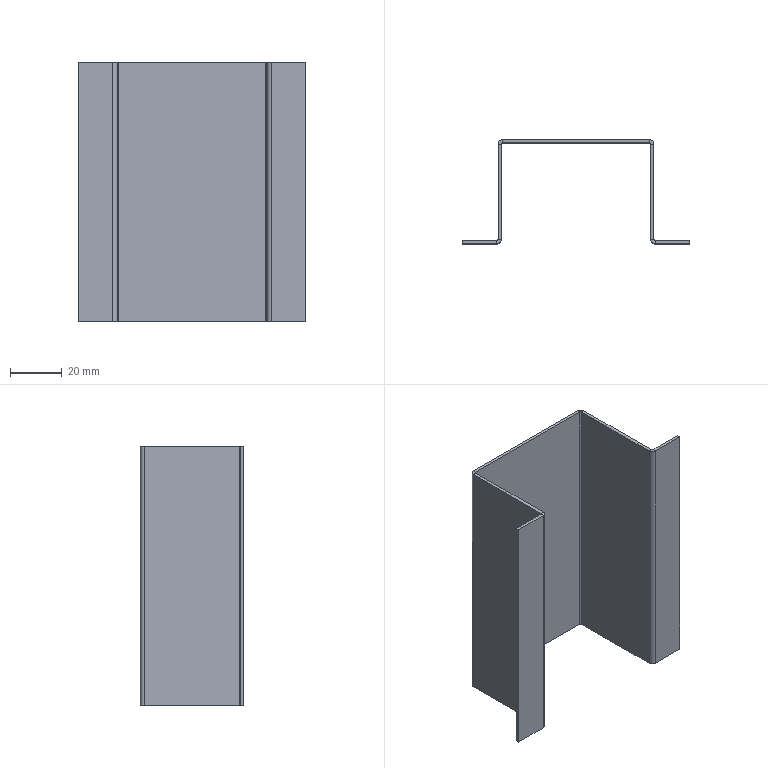Part | SolidWorks | features EdgeFlange 2, FlatPattern 1, SMBaseFlange 1, SheetMetal 1 | 1 solid | 38 faces | box 87.6 x 40 x 100 mm | volume 19608 mm3 | plane 30 | cylinder 8 | commonest cylinder face diameters 0.9 x4 3.3 x4
STEP:
#1=CARTESIAN_POINT('',(-19.132,-0.45,79.221));
#2=VERTEX_POINT('',#1);
#3=CARTESIAN_POINT('',(-19.132,-37.15,79.221));
#4=VERTEX_POINT('',#3);
#5=CARTESIAN_POINT('',(-19.132,-38.8,79.221));
#6=DIRECTION('',(0.,-1.,0.));
#7=VECTOR('',#6,1000.);
#8=LINE('',#5,#7);
#9=EDGE_CURVE('',#2,#4,#8,.T.);
#10=ORIENTED_EDGE('',*,*,#9,.T.);
#11=CARTESIAN_POINT('',(-17.932,-37.15,79.221));
#12=VERTEX_POINT('',#11);
#13=CARTESIAN_POINT('',(-19.132,-37.15,79.221));
#14=DIRECTION('',(1.,0.,0.));
#15=VECTOR('',#14,1000.);
#16=LINE('',#13,#15);
#17=EDGE_CURVE('',#4,#12,#16,.T.);
#18=ORIENTED_EDGE('',*,*,#17,.T.);
#19=CARTESIAN_POINT('',(-17.932,-0.45,79.221));
#20=VERTEX_POINT('',#19);
#21=CARTESIAN_POINT('',(-17.932,0.,79.221));
#22=DIRECTION('',(0.,-1.,0.));
#23=VECTOR('',#22,1000.);
#24=LINE('',#21,#23);
#25=EDGE_CURVE('',#20,#12,#24,.T.);
#26=ORIENTED_EDGE('',*,*,#25,.F.);
#27=CARTESIAN_POINT('',(-19.132,-0.45,79.221));
#28=DIRECTION('',(-1.,0.,0.));
#29=VECTOR('',#28,1000.);
#30=LINE('',#27,#29);
#31=EDGE_CURVE('',#20,#2,#30,.T.);
#32=ORIENTED_EDGE('',*,*,#31,.T.);
#33=EDGE_LOOP('',(#10,#18,#26,#32));
#34=FACE_OUTER_BOUND('',#33,.T.);
#35=CARTESIAN_POINT('',(-19.132,-38.8,79.221));
#36=DIRECTION('',(0.,0.,1.));
#37=DIRECTION('',(1.,0.,0.));
#38=AXIS2_PLACEMENT_3D('',#35,#36,#37);
#39=PLANE('',#38);
#40=ADVANCED_FACE('',(#34),#39,.T.);
#41=CARTESIAN_POINT('',(-19.132,-37.15,-20.779));
#42=VERTEX_POINT('',#41);
#43=CARTESIAN_POINT('',(-19.132,-0.45,-20.779));
#44=VERTEX_POINT('',#43);
#45=CARTESIAN_POINT('',(-19.132,0.,-20.779));
#46=DIRECTION('',(0.,1.,0.));
#47=VECTOR('',#46,1000.);
#48=LINE('',#45,#47);
#49=EDGE_CURVE('',#42,#44,#48,.T.);
#50=ORIENTED_EDGE('',*,*,#49,.F.);
#51=CARTESIAN_POINT('',(-19.132,-37.15,79.221));
#52=DIRECTION('',(0.,0.,-1.));
#53=VECTOR('',#52,1000.);
#54=LINE('',#51,#53);
#55=EDGE_CURVE('',#4,#42,#54,.T.);
#56=ORIENTED_EDGE('',*,*,#55,.F.);
#57=ORIENTED_EDGE('',*,*,#9,.F.);
#58=CARTESIAN_POINT('',(-19.132,-0.45,-20.779));
#59=DIRECTION('',(0.,0.,-1.));
#60=VECTOR('',#59,1000.);
#61=LINE('',#58,#60);
#62=EDGE_CURVE('',#2,#44,#61,.T.);
#63=ORIENTED_EDGE('',*,*,#62,.T.);
#64=EDGE_LOOP('',(#50,#56,#57,#63));
#65=FACE_OUTER_BOUND('',#64,.T.);
#66=CARTESIAN_POINT('',(-19.132,0.,-20.779));
#67=DIRECTION('',(-1.,0.,0.));
#68=DIRECTION('',(0.,-1.,0.));
#69=AXIS2_PLACEMENT_3D('',#66,#67,#68);
#70=PLANE('',#69);
#71=ADVANCED_FACE('',(#65),#70,.T.);
#72=CARTESIAN_POINT('',(-17.932,-37.15,-20.779));
#73=VERTEX_POINT('',#72);
#74=CARTESIAN_POINT('',(-17.932,-37.15,79.221));
#75=DIRECTION('',(0.,0.,-1.));
#76=VECTOR('',#75,1000.);
#77=LINE('',#74,#76);
#78=EDGE_CURVE('',#12,#73,#77,.T.);
#79=ORIENTED_EDGE('',*,*,#78,.T.);
#80=CARTESIAN_POINT('',(-17.932,-0.45,-20.779));
#81=VERTEX_POINT('',#80);
#82=CARTESIAN_POINT('',(-17.932,0.,-20.779));
#83=DIRECTION('',(0.,1.,0.));
#84=VECTOR('',#83,1000.);
#85=LINE('',#82,#84);
#86=EDGE_CURVE('',#73,#81,#85,.T.);
#87=ORIENTED_EDGE('',*,*,#86,.T.);
#88=CARTESIAN_POINT('',(-17.932,-0.45,79.221));
#89=DIRECTION('',(0.,0.,-1.));
#90=VECTOR('',#89,1000.);
#91=LINE('',#88,#90);
#92=EDGE_CURVE('',#20,#81,#91,.T.);
#93=ORIENTED_EDGE('',*,*,#92,.F.);
#94=ORIENTED_EDGE('',*,*,#25,.T.);
#95=EDGE_LOOP('',(#79,#87,#93,#94));
#96=FACE_OUTER_BOUND('',#95,.T.);
#97=CARTESIAN_POINT('',(-17.932,0.,-20.779));
#98=DIRECTION('',(-1.,0.,0.));
#99=DIRECTION('',(0.,-1.,0.));
#100=AXIS2_PLACEMENT_3D('',#97,#98,#99);
#101=PLANE('',#100);
#102=ADVANCED_FACE('',(#96),#101,.F.);
#103=CARTESIAN_POINT('',(40.868,-0.45,-20.779));
#104=VERTEX_POINT('',#103);
#105=CARTESIAN_POINT('',(40.868,-37.15,-20.779));
#106=VERTEX_POINT('',#105);
#107=CARTESIAN_POINT('',(40.868,0.,-20.779));
#108=DIRECTION('',(0.,-1.,0.));
#109=VECTOR('',#108,1000.);
#110=LINE('',#107,#109);
#111=EDGE_CURVE('',#104,#106,#110,.T.);
#112=ORIENTED_EDGE('',*,*,#111,.T.);
#113=CARTESIAN_POINT('',(39.668,-37.15,-20.779));
#114=VERTEX_POINT('',#113);
#115=CARTESIAN_POINT('',(40.868,-37.15,-20.779));
#116=DIRECTION('',(-1.,0.,0.));
#117=VECTOR('',#116,1000.);
#118=LINE('',#115,#117);
#119=EDGE_CURVE('',#106,#114,#118,.T.);
#120=ORIENTED_EDGE('',*,*,#119,.T.);
#121=CARTESIAN_POINT('',(39.668,-0.45,-20.779));
#122=VERTEX_POINT('',#121);
#123=CARTESIAN_POINT('',(39.668,-38.8,-20.779));
#124=DIRECTION('',(0.,-1.,0.));
#125=VECTOR('',#124,1000.);
#126=LINE('',#123,#125);
#127=EDGE_CURVE('',#122,#114,#126,.T.);
#128=ORIENTED_EDGE('',*,*,#127,.F.);
#129=CARTESIAN_POINT('',(40.868,-0.45,-20.779));
#130=DIRECTION('',(1.,0.,0.));
#131=VECTOR('',#130,1000.);
#132=LINE('',#129,#131);
#133=EDGE_CURVE('',#122,#104,#132,.T.);
#134=ORIENTED_EDGE('',*,*,#133,.T.);
#135=EDGE_LOOP('',(#112,#120,#128,#134));
#136=FACE_OUTER_BOUND('',#135,.T.);
#137=CARTESIAN_POINT('',(40.868,0.,-20.779));
#138=DIRECTION('',(0.,0.,-1.));
#139=DIRECTION('',(-1.,0.,0.));
#140=AXIS2_PLACEMENT_3D('',#137,#138,#139);
#141=PLANE('',#140);
#142=ADVANCED_FACE('',(#136),#141,.T.);
#143=CARTESIAN_POINT('',(40.868,-37.15,79.221));
#144=VERTEX_POINT('',#143);
#145=CARTESIAN_POINT('',(40.868,-37.15,-20.779));
#146=DIRECTION('',(0.,0.,1.));
#147=VECTOR('',#146,1000.);
#148=LINE('',#145,#147);
#149=EDGE_CURVE('',#106,#144,#148,.T.);
#150=ORIENTED_EDGE('',*,*,#149,.F.);
#151=ORIENTED_EDGE('',*,*,#111,.F.);
#152=CARTESIAN_POINT('',(40.868,-0.45,79.221));
#153=VERTEX_POINT('',#152);
#154=CARTESIAN_POINT('',(40.868,-0.45,-20.779));
#155=DIRECTION('',(0.,0.,-1.));
#156=VECTOR('',#155,1000.);
#157=LINE('',#154,#156);
#158=EDGE_CURVE('',#153,#104,#157,.T.);
#159=ORIENTED_EDGE('',*,*,#158,.F.);
#160=CARTESIAN_POINT('',(40.868,-38.8,79.221));
#161=DIRECTION('',(0.,1.,0.));
#162=VECTOR('',#161,1000.);
#163=LINE('',#160,#162);
#164=EDGE_CURVE('',#144,#153,#163,.T.);
#165=ORIENTED_EDGE('',*,*,#164,.F.);
#166=EDGE_LOOP('',(#150,#151,#159,#165));
#167=FACE_OUTER_BOUND('',#166,.T.);
#168=CARTESIAN_POINT('',(40.868,-38.8,-20.779));
#169=DIRECTION('',(-1.,0.,0.));
#170=DIRECTION('',(0.,-1.,0.));
#171=AXIS2_PLACEMENT_3D('',#168,#169,#170);
#172=PLANE('',#171);
#173=ADVANCED_FACE('',(#167),#172,.F.);
#174=ORIENTED_EDGE('',*,*,#127,.T.);
#175=CARTESIAN_POINT('',(39.668,-37.15,79.221));
#176=VERTEX_POINT('',#175);
#177=CARTESIAN_POINT('',(39.668,-37.15,-20.779));
#178=DIRECTION('',(0.,0.,1.));
#179=VECTOR('',#178,1000.);
#180=LINE('',#177,#179);
#181=EDGE_CURVE('',#114,#176,#180,.T.);
#182=ORIENTED_EDGE('',*,*,#181,.T.);
#183=CARTESIAN_POINT('',(39.668,-0.45,79.221));
#184=VERTEX_POINT('',#183);
#185=CARTESIAN_POINT('',(39.668,-38.8,79.221));
#186=DIRECTION('',(0.,1.,0.));
#187=VECTOR('',#186,1000.);
#188=LINE('',#185,#187);
#189=EDGE_CURVE('',#176,#184,#188,.T.);
#190=ORIENTED_EDGE('',*,*,#189,.T.);
#191=CARTESIAN_POINT('',(39.668,-0.45,-20.779));
#192=DIRECTION('',(0.,0.,1.));
#193=VECTOR('',#192,1000.);
#194=LINE('',#191,#193);
#195=EDGE_CURVE('',#122,#184,#194,.T.);
#196=ORIENTED_EDGE('',*,*,#195,.F.);
#197=EDGE_LOOP('',(#174,#182,#190,#196));
#198=FACE_OUTER_BOUND('',#197,.T.);
#199=CARTESIAN_POINT('',(39.668,-38.8,-20.779));
#200=DIRECTION('',(-1.,0.,0.));
#201=DIRECTION('',(0.,-1.,0.));
#202=AXIS2_PLACEMENT_3D('',#199,#200,#201);
#203=PLANE('',#202);
#204=ADVANCED_FACE('',(#198),#203,.T.);
#205=CARTESIAN_POINT('',(39.218,0.,79.221));
#206=VERTEX_POINT('',#205);
#207=CARTESIAN_POINT('',(39.218,1.2,79.221));
#208=VERTEX_POINT('',#207);
#209=CARTESIAN_POINT('',(39.218,0.,79.221));
#210=DIRECTION('',(0.,1.,0.));
#211=VECTOR('',#210,1000.);
#212=LINE('',#209,#211);
#213=EDGE_CURVE('',#206,#208,#212,.T.);
#214=ORIENTED_EDGE('',*,*,#213,.T.);
#215=CARTESIAN_POINT('',(-17.482,1.2,79.221));
#216=VERTEX_POINT('',#215);
#217=CARTESIAN_POINT('',(-19.132,1.2,79.221));
#218=DIRECTION('',(1.,0.,0.));
#219=VECTOR('',#218,1000.);
#220=LINE('',#217,#219);
#221=EDGE_CURVE('',#216,#208,#220,.T.);
#222=ORIENTED_EDGE('',*,*,#221,.F.);
#223=CARTESIAN_POINT('',(-17.482,0.,79.221));
#224=VERTEX_POINT('',#223);
#225=CARTESIAN_POINT('',(-17.482,0.,79.221));
#226=DIRECTION('',(0.,1.,0.));
#227=VECTOR('',#226,1000.);
#228=LINE('',#225,#227);
#229=EDGE_CURVE('',#224,#216,#228,.T.);
#230=ORIENTED_EDGE('',*,*,#229,.F.);
#231=CARTESIAN_POINT('',(-19.132,0.,79.221));
#232=DIRECTION('',(1.,0.,0.));
#233=VECTOR('',#232,1000.);
#234=LINE('',#231,#233);
#235=EDGE_CURVE('',#224,#206,#234,.T.);
#236=ORIENTED_EDGE('',*,*,#235,.T.);
#237=EDGE_LOOP('',(#214,#222,#230,#236));
#238=FACE_OUTER_BOUND('',#237,.T.);
#239=CARTESIAN_POINT('',(-19.132,1.2,79.221));
#240=DIRECTION('',(0.,0.,-1.));
#241=DIRECTION('',(-1.,0.,0.));
#242=AXIS2_PLACEMENT_3D('',#239,#240,#241);
#243=PLANE('',#242);
#244=ADVANCED_FACE('',(#238),#243,.F.);
#245=CARTESIAN_POINT('',(39.218,0.,-20.779));
#246=VERTEX_POINT('',#245);
#247=CARTESIAN_POINT('',(39.218,1.2,-20.779));
#248=VERTEX_POINT('',#247);
#249=CARTESIAN_POINT('',(39.218,0.,-20.779));
#250=DIRECTION('',(0.,1.,0.));
#251=VECTOR('',#250,1000.);
#252=LINE('',#249,#251);
#253=EDGE_CURVE('',#246,#248,#252,.T.);
#254=ORIENTED_EDGE('',*,*,#253,.F.);
#255=CARTESIAN_POINT('',(-17.482,0.,-20.779));
#256=VERTEX_POINT('',#255);
#257=CARTESIAN_POINT('',(-19.132,0.,-20.779));
#258=DIRECTION('',(-1.,0.,0.));
#259=VECTOR('',#258,1000.);
#260=LINE('',#257,#259);
#261=EDGE_CURVE('',#246,#256,#260,.T.);
#262=ORIENTED_EDGE('',*,*,#261,.T.);
#263=CARTESIAN_POINT('',(-17.482,1.2,-20.779));
#264=VERTEX_POINT('',#263);
#265=CARTESIAN_POINT('',(-17.482,0.,-20.779));
#266=DIRECTION('',(0.,1.,0.));
#267=VECTOR('',#266,1000.);
#268=LINE('',#265,#267);
#269=EDGE_CURVE('',#256,#264,#268,.T.);
#270=ORIENTED_EDGE('',*,*,#269,.T.);
#271=CARTESIAN_POINT('',(-19.132,1.2,-20.779));
#272=DIRECTION('',(-1.,0.,0.));
#273=VECTOR('',#272,1000.);
#274=LINE('',#271,#273);
#275=EDGE_CURVE('',#248,#264,#274,.T.);
#276=ORIENTED_EDGE('',*,*,#275,.F.);
#277=EDGE_LOOP('',(#254,#262,#270,#276));
#278=FACE_OUTER_BOUND('',#277,.T.);
#279=CARTESIAN_POINT('',(-19.132,1.2,-20.779));
#280=DIRECTION('',(0.,0.,1.));
#281=DIRECTION('',(1.,0.,0.));
#282=AXIS2_PLACEMENT_3D('',#279,#280,#281);
#283=PLANE('',#282);
#284=ADVANCED_FACE('',(#278),#283,.F.);
#285=ORIENTED_EDGE('',*,*,#221,.T.);
#286=CARTESIAN_POINT('',(39.218,1.2,79.221));
#287=DIRECTION('',(0.,0.,-1.));
#288=VECTOR('',#287,1000.);
#289=LINE('',#286,#288);
#290=EDGE_CURVE('',#208,#248,#289,.T.);
#291=ORIENTED_EDGE('',*,*,#290,.T.);
#292=ORIENTED_EDGE('',*,*,#275,.T.);
#293=CARTESIAN_POINT('',(-17.482,1.2,-20.779));
#294=DIRECTION('',(0.,0.,1.));
#295=VECTOR('',#294,1000.);
#296=LINE('',#293,#295);
#297=EDGE_CURVE('',#264,#216,#296,.T.);
#298=ORIENTED_EDGE('',*,*,#297,.T.);
#299=EDGE_LOOP('',(#285,#291,#292,#298));
#300=FACE_OUTER_BOUND('',#299,.T.);
#301=CARTESIAN_POINT('',(-19.132,1.2,79.221));
#302=DIRECTION('',(0.,1.,0.));
#303=DIRECTION('',(0.,0.,1.));
#304=AXIS2_PLACEMENT_3D('',#301,#302,#303);
#305=PLANE('',#304);
#306=ADVANCED_FACE('',(#300),#305,.T.);
#307=CARTESIAN_POINT('',(39.218,0.,79.221));
#308=DIRECTION('',(0.,0.,-1.));
#309=VECTOR('',#308,1000.);
#310=LINE('',#307,#309);
#311=EDGE_CURVE('',#206,#246,#310,.T.);
#312=ORIENTED_EDGE('',*,*,#311,.F.);
#313=ORIENTED_EDGE('',*,*,#235,.F.);
#314=CARTESIAN_POINT('',(-17.482,0.,-20.779));
#315=DIRECTION('',(0.,0.,1.));
#316=VECTOR('',#315,1000.);
#317=LINE('',#314,#316);
#318=EDGE_CURVE('',#256,#224,#317,.T.);
#319=ORIENTED_EDGE('',*,*,#318,.F.);
#320=ORIENTED_EDGE('',*,*,#261,.F.);
#321=EDGE_LOOP('',(#312,#313,#319,#320));
#322=FACE_OUTER_BOUND('',#321,.T.);
#323=CARTESIAN_POINT('',(-19.132,0.,79.221));
#324=DIRECTION('',(0.,1.,0.));
#325=DIRECTION('',(0.,0.,1.));
#326=AXIS2_PLACEMENT_3D('',#323,#324,#325);
#327=PLANE('',#326);
#328=ADVANCED_FACE('',(#322),#327,.F.);
#329=ORIENTED_EDGE('',*,*,#31,.F.);
#330=CARTESIAN_POINT('',(-17.482,-0.45,79.221));
#331=DIRECTION('',(0.,0.,1.));
#332=DIRECTION('',(-1.,0.,0.));
#333=AXIS2_PLACEMENT_3D('',#330,#331,#332);
#334=CIRCLE('',#333,0.45);
#335=EDGE_CURVE('',#224,#20,#334,.T.);
#336=ORIENTED_EDGE('',*,*,#335,.F.);
#337=ORIENTED_EDGE('',*,*,#229,.T.);
#338=CARTESIAN_POINT('',(-17.482,-0.45,79.221));
#339=DIRECTION('',(0.,0.,1.));
#340=DIRECTION('',(-1.,0.,0.));
#341=AXIS2_PLACEMENT_3D('',#338,#339,#340);
#342=CIRCLE('',#341,1.65);
#343=EDGE_CURVE('',#216,#2,#342,.T.);
#344=ORIENTED_EDGE('',*,*,#343,.T.);
#345=EDGE_LOOP('',(#329,#336,#337,#344));
#346=FACE_OUTER_BOUND('',#345,.T.);
#347=CARTESIAN_POINT('',(-17.482,-0.45,79.221));
#348=DIRECTION('',(0.,0.,1.));
#349=DIRECTION('',(1.,0.,0.));
#350=AXIS2_PLACEMENT_3D('',#347,#348,#349);
#351=PLANE('',#350);
#352=ADVANCED_FACE('',(#346),#351,.T.);
#353=ORIENTED_EDGE('',*,*,#297,.F.);
#354=CARTESIAN_POINT('',(-17.482,-0.45,-20.779));
#355=DIRECTION('',(0.,0.,-1.));
#356=DIRECTION('',(-1.,0.,0.));
#357=AXIS2_PLACEMENT_3D('',#354,#355,#356);
#358=CIRCLE('',#357,1.65);
#359=EDGE_CURVE('',#44,#264,#358,.T.);
#360=ORIENTED_EDGE('',*,*,#359,.F.);
#361=ORIENTED_EDGE('',*,*,#62,.F.);
#362=ORIENTED_EDGE('',*,*,#343,.F.);
#363=EDGE_LOOP('',(#353,#360,#361,#362));
#364=FACE_OUTER_BOUND('',#363,.T.);
#365=CARTESIAN_POINT('',(-17.482,-0.45,-20.779));
#366=DIRECTION('',(0.,0.,-1.));
#367=DIRECTION('',(-1.,0.,0.));
#368=AXIS2_PLACEMENT_3D('',#365,#366,#367);
#369=CYLINDRICAL_SURFACE('',#368,1.65);
#370=ADVANCED_FACE('',(#364),#369,.T.);
#371=CARTESIAN_POINT('',(-17.482,-0.45,-20.779));
#372=DIRECTION('',(0.,0.,-1.));
#373=DIRECTION('',(-1.,0.,0.));
#374=AXIS2_PLACEMENT_3D('',#371,#372,#373);
#375=CIRCLE('',#374,0.45);
#376=EDGE_CURVE('',#81,#256,#375,.T.);
#377=ORIENTED_EDGE('',*,*,#376,.F.);
#378=CARTESIAN_POINT('',(-17.932,-0.45,-20.779));
#379=DIRECTION('',(-1.,0.,0.));
#380=VECTOR('',#379,1000.);
#381=LINE('',#378,#380);
#382=EDGE_CURVE('',#81,#44,#381,.T.);
#383=ORIENTED_EDGE('',*,*,#382,.T.);
#384=ORIENTED_EDGE('',*,*,#359,.T.);
#385=ORIENTED_EDGE('',*,*,#269,.F.);
#386=EDGE_LOOP('',(#377,#383,#384,#385));
#387=FACE_OUTER_BOUND('',#386,.T.);
#388=CARTESIAN_POINT('',(-17.482,-0.45,-20.779));
#389=DIRECTION('',(0.,0.,1.));
#390=DIRECTION('',(1.,0.,0.));
#391=AXIS2_PLACEMENT_3D('',#388,#389,#390);
#392=PLANE('',#391);
#393=ADVANCED_FACE('',(#387),#392,.F.);
#394=ORIENTED_EDGE('',*,*,#318,.T.);
#395=ORIENTED_EDGE('',*,*,#335,.T.);
#396=ORIENTED_EDGE('',*,*,#92,.T.);
#397=ORIENTED_EDGE('',*,*,#376,.T.);
#398=EDGE_LOOP('',(#394,#395,#396,#397));
#399=FACE_OUTER_BOUND('',#398,.T.);
#400=CARTESIAN_POINT('',(-17.482,-0.45,-20.779));
#401=DIRECTION('',(0.,0.,-1.));
#402=DIRECTION('',(-1.,0.,0.));
#403=AXIS2_PLACEMENT_3D('',#400,#401,#402);
#404=CYLINDRICAL_SURFACE('',#403,0.45);
#405=ADVANCED_FACE('',(#399),#404,.F.);
#406=CARTESIAN_POINT('',(-19.132,-37.15,-20.779));
#407=DIRECTION('',(1.,0.,0.));
#408=VECTOR('',#407,1000.);
#409=LINE('',#406,#408);
#410=EDGE_CURVE('',#42,#73,#409,.T.);
#411=ORIENTED_EDGE('',*,*,#410,.F.);
#412=ORIENTED_EDGE('',*,*,#49,.T.);
#413=ORIENTED_EDGE('',*,*,#382,.F.);
#414=ORIENTED_EDGE('',*,*,#86,.F.);
#415=EDGE_LOOP('',(#411,#412,#413,#414));
#416=FACE_OUTER_BOUND('',#415,.T.);
#417=CARTESIAN_POINT('',(-19.132,0.,-20.779));
#418=DIRECTION('',(0.,0.,-1.));
#419=DIRECTION('',(-1.,0.,0.));
#420=AXIS2_PLACEMENT_3D('',#417,#418,#419);
#421=PLANE('',#420);
#422=ADVANCED_FACE('',(#416),#421,.T.);
#423=ORIENTED_EDGE('',*,*,#133,.F.);
#424=CARTESIAN_POINT('',(39.218,-0.45,-20.779));
#425=DIRECTION('',(0.,0.,-1.));
#426=DIRECTION('',(1.,0.,0.));
#427=AXIS2_PLACEMENT_3D('',#424,#425,#426);
#428=CIRCLE('',#427,0.45);
#429=EDGE_CURVE('',#246,#122,#428,.T.);
#430=ORIENTED_EDGE('',*,*,#429,.F.);
#431=ORIENTED_EDGE('',*,*,#253,.T.);
#432=CARTESIAN_POINT('',(39.218,-0.45,-20.779));
#433=DIRECTION('',(0.,0.,-1.));
#434=DIRECTION('',(1.,0.,0.));
#435=AXIS2_PLACEMENT_3D('',#432,#433,#434);
#436=CIRCLE('',#435,1.65);
#437=EDGE_CURVE('',#248,#104,#436,.T.);
#438=ORIENTED_EDGE('',*,*,#437,.T.);
#439=EDGE_LOOP('',(#423,#430,#431,#438));
#440=FACE_OUTER_BOUND('',#439,.T.);
#441=CARTESIAN_POINT('',(39.218,-0.45,-20.779));
#442=DIRECTION('',(0.,0.,-1.));
#443=DIRECTION('',(-1.,0.,0.));
#444=AXIS2_PLACEMENT_3D('',#441,#442,#443);
#445=PLANE('',#444);
#446=ADVANCED_FACE('',(#440),#445,.T.);
#447=ORIENTED_EDGE('',*,*,#290,.F.);
#448=CARTESIAN_POINT('',(39.218,-0.45,79.221));
#449=DIRECTION('',(0.,0.,1.));
#450=DIRECTION('',(1.,0.,0.));
#451=AXIS2_PLACEMENT_3D('',#448,#449,#450);
#452=CIRCLE('',#451,1.65);
#453=EDGE_CURVE('',#153,#208,#452,.T.);
#454=ORIENTED_EDGE('',*,*,#453,.F.);
#455=ORIENTED_EDGE('',*,*,#158,.T.);
#456=ORIENTED_EDGE('',*,*,#437,.F.);
#457=EDGE_LOOP('',(#447,#454,#455,#456));
#458=FACE_OUTER_BOUND('',#457,.T.);
#459=CARTESIAN_POINT('',(39.218,-0.45,79.221));
#460=DIRECTION('',(0.,0.,1.));
#461=DIRECTION('',(1.,0.,0.));
#462=AXIS2_PLACEMENT_3D('',#459,#460,#461);
#463=CYLINDRICAL_SURFACE('',#462,1.65);
#464=ADVANCED_FACE('',(#458),#463,.T.);
#465=CARTESIAN_POINT('',(39.218,-0.45,79.221));
#466=DIRECTION('',(0.,0.,1.));
#467=DIRECTION('',(1.,0.,0.));
#468=AXIS2_PLACEMENT_3D('',#465,#466,#467);
#469=CIRCLE('',#468,0.45);
#470=EDGE_CURVE('',#184,#206,#469,.T.);
#471=ORIENTED_EDGE('',*,*,#470,.F.);
#472=CARTESIAN_POINT('',(39.668,-0.45,79.221));
#473=DIRECTION('',(1.,0.,0.));
#474=VECTOR('',#473,1000.);
#475=LINE('',#472,#474);
#476=EDGE_CURVE('',#184,#153,#475,.T.);
#477=ORIENTED_EDGE('',*,*,#476,.T.);
#478=ORIENTED_EDGE('',*,*,#453,.T.);
#479=ORIENTED_EDGE('',*,*,#213,.F.);
#480=EDGE_LOOP('',(#471,#477,#478,#479));
#481=FACE_OUTER_BOUND('',#480,.T.);
#482=CARTESIAN_POINT('',(39.218,-0.45,79.221));
#483=DIRECTION('',(0.,0.,-1.));
#484=DIRECTION('',(-1.,0.,0.));
#485=AXIS2_PLACEMENT_3D('',#482,#483,#484);
#486=PLANE('',#485);
#487=ADVANCED_FACE('',(#481),#486,.F.);
#488=ORIENTED_EDGE('',*,*,#311,.T.);
#489=ORIENTED_EDGE('',*,*,#429,.T.);
#490=ORIENTED_EDGE('',*,*,#195,.T.);
#491=ORIENTED_EDGE('',*,*,#470,.T.);
#492=EDGE_LOOP('',(#488,#489,#490,#491));
#493=FACE_OUTER_BOUND('',#492,.T.);
#494=CARTESIAN_POINT('',(39.218,-0.45,79.221));
#495=DIRECTION('',(0.,0.,1.));
#496=DIRECTION('',(1.,0.,0.));
#497=AXIS2_PLACEMENT_3D('',#494,#495,#496);
#498=CYLINDRICAL_SURFACE('',#497,0.45);
#499=ADVANCED_FACE('',(#493),#498,.F.);
#500=CARTESIAN_POINT('',(40.868,-37.15,79.221));
#501=DIRECTION('',(-1.,0.,0.));
#502=VECTOR('',#501,1000.);
#503=LINE('',#500,#502);
#504=EDGE_CURVE('',#144,#176,#503,.T.);
#505=ORIENTED_EDGE('',*,*,#504,.F.);
#506=ORIENTED_EDGE('',*,*,#164,.T.);
#507=ORIENTED_EDGE('',*,*,#476,.F.);
#508=ORIENTED_EDGE('',*,*,#189,.F.);
#509=EDGE_LOOP('',(#505,#506,#507,#508));
#510=FACE_OUTER_BOUND('',#509,.T.);
#511=CARTESIAN_POINT('',(40.868,-38.8,79.221));
#512=DIRECTION('',(0.,0.,1.));
#513=DIRECTION('',(1.,0.,0.));
#514=AXIS2_PLACEMENT_3D('',#511,#512,#513);
#515=PLANE('',#514);
#516=ADVANCED_FACE('',(#510),#515,.T.);
#517=CARTESIAN_POINT('',(41.318,-37.6,79.221));
#518=VERTEX_POINT('',#517);
#519=CARTESIAN_POINT('',(41.318,-38.8,79.221));
#520=VERTEX_POINT('',#519);
#521=CARTESIAN_POINT('',(41.318,-38.8,79.221));
#522=DIRECTION('',(0.,-1.,0.));
#523=VECTOR('',#522,1000.);
#524=LINE('',#521,#523);
#525=EDGE_CURVE('',#518,#520,#524,.T.);
#526=ORIENTED_EDGE('',*,*,#525,.F.);
#527=CARTESIAN_POINT('',(41.318,-37.15,79.221));
#528=DIRECTION('',(0.,0.,1.));
#529=DIRECTION('',(-1.,0.,0.));
#530=AXIS2_PLACEMENT_3D('',#527,#528,#529);
#531=CIRCLE('',#530,0.45);
#532=EDGE_CURVE('',#144,#518,#531,.T.);
#533=ORIENTED_EDGE('',*,*,#532,.F.);
#534=ORIENTED_EDGE('',*,*,#504,.T.);
#535=CARTESIAN_POINT('',(41.318,-37.15,79.221));
#536=DIRECTION('',(0.,0.,1.));
#537=DIRECTION('',(-1.,0.,0.));
#538=AXIS2_PLACEMENT_3D('',#535,#536,#537);
#539=CIRCLE('',#538,1.65);
#540=EDGE_CURVE('',#176,#520,#539,.T.);
#541=ORIENTED_EDGE('',*,*,#540,.T.);
#542=EDGE_LOOP('',(#526,#533,#534,#541));
#543=FACE_OUTER_BOUND('',#542,.T.);
#544=CARTESIAN_POINT('',(41.318,-37.15,79.221));
#545=DIRECTION('',(0.,0.,1.));
#546=DIRECTION('',(1.,0.,0.));
#547=AXIS2_PLACEMENT_3D('',#544,#545,#546);
#548=PLANE('',#547);
#549=ADVANCED_FACE('',(#543),#548,.T.);
#550=ORIENTED_EDGE('',*,*,#181,.F.);
#551=CARTESIAN_POINT('',(41.318,-38.8,-20.779));
#552=VERTEX_POINT('',#551);
#553=CARTESIAN_POINT('',(41.318,-37.15,-20.779));
#554=DIRECTION('',(0.,0.,-1.));
#555=DIRECTION('',(-1.,0.,0.));
#556=AXIS2_PLACEMENT_3D('',#553,#554,#555);
#557=CIRCLE('',#556,1.65);
#558=EDGE_CURVE('',#552,#114,#557,.T.);
#559=ORIENTED_EDGE('',*,*,#558,.F.);
#560=CARTESIAN_POINT('',(41.318,-38.8,79.221));
#561=DIRECTION('',(0.,0.,1.));
#562=VECTOR('',#561,1000.);
#563=LINE('',#560,#562);
#564=EDGE_CURVE('',#552,#520,#563,.T.);
#565=ORIENTED_EDGE('',*,*,#564,.T.);
#566=ORIENTED_EDGE('',*,*,#540,.F.);
#567=EDGE_LOOP('',(#550,#559,#565,#566));
#568=FACE_OUTER_BOUND('',#567,.T.);
#569=CARTESIAN_POINT('',(41.318,-37.15,-20.779));
#570=DIRECTION('',(0.,0.,-1.));
#571=DIRECTION('',(0.,-1.,0.));
#572=AXIS2_PLACEMENT_3D('',#569,#570,#571);
#573=CYLINDRICAL_SURFACE('',#572,1.65);
#574=ADVANCED_FACE('',(#568),#573,.T.);
#575=CARTESIAN_POINT('',(41.318,-37.6,-20.779));
#576=VERTEX_POINT('',#575);
#577=CARTESIAN_POINT('',(41.318,-37.15,-20.779));
#578=DIRECTION('',(0.,0.,-1.));
#579=DIRECTION('',(-1.,0.,0.));
#580=AXIS2_PLACEMENT_3D('',#577,#578,#579);
#581=CIRCLE('',#580,0.45);
#582=EDGE_CURVE('',#576,#106,#581,.T.);
#583=ORIENTED_EDGE('',*,*,#582,.F.);
#584=CARTESIAN_POINT('',(41.318,-37.6,-20.779));
#585=DIRECTION('',(0.,-1.,0.));
#586=VECTOR('',#585,1000.);
#587=LINE('',#584,#586);
#588=EDGE_CURVE('',#576,#552,#587,.T.);
#589=ORIENTED_EDGE('',*,*,#588,.T.);
#590=ORIENTED_EDGE('',*,*,#558,.T.);
#591=ORIENTED_EDGE('',*,*,#119,.F.);
#592=EDGE_LOOP('',(#583,#589,#590,#591));
#593=FACE_OUTER_BOUND('',#592,.T.);
#594=CARTESIAN_POINT('',(41.318,-37.15,-20.779));
#595=DIRECTION('',(0.,0.,1.));
#596=DIRECTION('',(1.,0.,0.));
#597=AXIS2_PLACEMENT_3D('',#594,#595,#596);
#598=PLANE('',#597);
#599=ADVANCED_FACE('',(#593),#598,.F.);
#600=ORIENTED_EDGE('',*,*,#149,.T.);
#601=ORIENTED_EDGE('',*,*,#532,.T.);
#602=CARTESIAN_POINT('',(41.318,-37.6,79.221));
#603=DIRECTION('',(0.,0.,-1.));
#604=VECTOR('',#603,1000.);
#605=LINE('',#602,#604);
#606=EDGE_CURVE('',#518,#576,#605,.T.);
#607=ORIENTED_EDGE('',*,*,#606,.T.);
#608=ORIENTED_EDGE('',*,*,#582,.T.);
#609=EDGE_LOOP('',(#600,#601,#607,#608));
#610=FACE_OUTER_BOUND('',#609,.T.);
#611=CARTESIAN_POINT('',(41.318,-37.15,-20.779));
#612=DIRECTION('',(0.,0.,-1.));
#613=DIRECTION('',(0.,-1.,0.));
#614=AXIS2_PLACEMENT_3D('',#611,#612,#613);
#615=CYLINDRICAL_SURFACE('',#614,0.45);
#616=ADVANCED_FACE('',(#610),#615,.F.);
#617=ORIENTED_EDGE('',*,*,#588,.F.);
#618=CARTESIAN_POINT('',(54.668,-37.6,-20.779));
#619=VERTEX_POINT('',#618);
#620=CARTESIAN_POINT('',(54.668,-37.6,-20.779));
#621=DIRECTION('',(1.,0.,0.));
#622=VECTOR('',#621,1000.);
#623=LINE('',#620,#622);
#624=EDGE_CURVE('',#576,#619,#623,.T.);
#625=ORIENTED_EDGE('',*,*,#624,.T.);
#626=CARTESIAN_POINT('',(54.668,-38.8,-20.779));
#627=VERTEX_POINT('',#626);
#628=CARTESIAN_POINT('',(54.668,-38.8,-20.779));
#629=DIRECTION('',(0.,1.,0.));
#630=VECTOR('',#629,1000.);
#631=LINE('',#628,#630);
#632=EDGE_CURVE('',#627,#619,#631,.T.);
#633=ORIENTED_EDGE('',*,*,#632,.F.);
#634=CARTESIAN_POINT('',(40.868,-38.8,-20.779));
#635=DIRECTION('',(1.,0.,0.));
#636=VECTOR('',#635,1000.);
#637=LINE('',#634,#636);
#638=EDGE_CURVE('',#552,#627,#637,.T.);
#639=ORIENTED_EDGE('',*,*,#638,.F.);
#640=EDGE_LOOP('',(#617,#625,#633,#639));
#641=FACE_OUTER_BOUND('',#640,.T.);
#642=CARTESIAN_POINT('',(54.668,-38.8,-20.779));
#643=DIRECTION('',(0.,0.,1.));
#644=DIRECTION('',(0.,-1.,0.));
#645=AXIS2_PLACEMENT_3D('',#642,#643,#644);
#646=PLANE('',#645);
#647=ADVANCED_FACE('',(#641),#646,.F.);
#648=ORIENTED_EDGE('',*,*,#525,.T.);
#649=CARTESIAN_POINT('',(54.668,-38.8,79.221));
#650=VERTEX_POINT('',#649);
#651=CARTESIAN_POINT('',(40.868,-38.8,79.221));
#652=DIRECTION('',(-1.,0.,0.));
#653=VECTOR('',#652,1000.);
#654=LINE('',#651,#653);
#655=EDGE_CURVE('',#650,#520,#654,.T.);
#656=ORIENTED_EDGE('',*,*,#655,.F.);
#657=CARTESIAN_POINT('',(54.668,-37.6,79.221));
#658=VERTEX_POINT('',#657);
#659=CARTESIAN_POINT('',(54.668,-38.8,79.221));
#660=DIRECTION('',(0.,1.,0.));
#661=VECTOR('',#660,1000.);
#662=LINE('',#659,#661);
#663=EDGE_CURVE('',#650,#658,#662,.T.);
#664=ORIENTED_EDGE('',*,*,#663,.T.);
#665=CARTESIAN_POINT('',(40.868,-37.6,79.221));
#666=DIRECTION('',(-1.,0.,0.));
#667=VECTOR('',#666,1000.);
#668=LINE('',#665,#667);
#669=EDGE_CURVE('',#658,#518,#668,.T.);
#670=ORIENTED_EDGE('',*,*,#669,.T.);
#671=EDGE_LOOP('',(#648,#656,#664,#670));
#672=FACE_OUTER_BOUND('',#671,.T.);
#673=CARTESIAN_POINT('',(40.868,-38.8,79.221));
#674=DIRECTION('',(0.,0.,-1.));
#675=DIRECTION('',(0.,1.,0.));
#676=AXIS2_PLACEMENT_3D('',#673,#674,#675);
#677=PLANE('',#676);
#678=ADVANCED_FACE('',(#672),#677,.F.);
#679=ORIENTED_EDGE('',*,*,#564,.F.);
#680=ORIENTED_EDGE('',*,*,#638,.T.);
#681=CARTESIAN_POINT('',(54.668,-38.8,-20.779));
#682=DIRECTION('',(0.,0.,1.));
#683=VECTOR('',#682,1000.);
#684=LINE('',#681,#683);
#685=EDGE_CURVE('',#627,#650,#684,.T.);
#686=ORIENTED_EDGE('',*,*,#685,.T.);
#687=ORIENTED_EDGE('',*,*,#655,.T.);
#688=EDGE_LOOP('',(#679,#680,#686,#687));
#689=FACE_OUTER_BOUND('',#688,.T.);
#690=CARTESIAN_POINT('',(40.868,-38.8,-20.779));
#691=DIRECTION('',(0.,1.,0.));
#692=DIRECTION('',(0.,0.,1.));
#693=AXIS2_PLACEMENT_3D('',#690,#691,#692);
#694=PLANE('',#693);
#695=ADVANCED_FACE('',(#689),#694,.F.);
#696=ORIENTED_EDGE('',*,*,#624,.F.);
#697=ORIENTED_EDGE('',*,*,#606,.F.);
#698=ORIENTED_EDGE('',*,*,#669,.F.);
#699=CARTESIAN_POINT('',(54.668,-37.6,79.221));
#700=DIRECTION('',(0.,0.,1.));
#701=VECTOR('',#700,1000.);
#702=LINE('',#699,#701);
#703=EDGE_CURVE('',#619,#658,#702,.T.);
#704=ORIENTED_EDGE('',*,*,#703,.F.);
#705=EDGE_LOOP('',(#696,#697,#698,#704));
#706=FACE_OUTER_BOUND('',#705,.T.);
#707=CARTESIAN_POINT('',(40.868,-37.6,-20.779));
#708=DIRECTION('',(0.,1.,0.));
#709=DIRECTION('',(0.,0.,1.));
#710=AXIS2_PLACEMENT_3D('',#707,#708,#709);
#711=PLANE('',#710);
#712=ADVANCED_FACE('',(#706),#711,.T.);
#713=ORIENTED_EDGE('',*,*,#703,.T.);
#714=ORIENTED_EDGE('',*,*,#663,.F.);
#715=ORIENTED_EDGE('',*,*,#685,.F.);
#716=ORIENTED_EDGE('',*,*,#632,.T.);
#717=EDGE_LOOP('',(#713,#714,#715,#716));
#718=FACE_OUTER_BOUND('',#717,.T.);
#719=CARTESIAN_POINT('',(54.668,-38.8,79.221));
#720=DIRECTION('',(-1.,0.,0.));
#721=DIRECTION('',(0.,0.,1.));
#722=AXIS2_PLACEMENT_3D('',#719,#720,#721);
#723=PLANE('',#722);
#724=ADVANCED_FACE('',(#718),#723,.F.);
#725=CARTESIAN_POINT('',(-19.582,-37.6,-20.779));
#726=VERTEX_POINT('',#725);
#727=CARTESIAN_POINT('',(-19.582,-38.8,-20.779));
#728=VERTEX_POINT('',#727);
#729=CARTESIAN_POINT('',(-19.582,-38.8,-20.779));
#730=DIRECTION('',(0.,-1.,0.));
#731=VECTOR('',#730,1000.);
#732=LINE('',#729,#731);
#733=EDGE_CURVE('',#726,#728,#732,.T.);
#734=ORIENTED_EDGE('',*,*,#733,.F.);
#735=CARTESIAN_POINT('',(-19.582,-37.15,-20.779));
#736=DIRECTION('',(0.,0.,-1.));
#737=DIRECTION('',(1.,0.,0.));
#738=AXIS2_PLACEMENT_3D('',#735,#736,#737);
#739=CIRCLE('',#738,0.45);
#740=EDGE_CURVE('',#42,#726,#739,.T.);
#741=ORIENTED_EDGE('',*,*,#740,.F.);
#742=ORIENTED_EDGE('',*,*,#410,.T.);
#743=CARTESIAN_POINT('',(-19.582,-37.15,-20.779));
#744=DIRECTION('',(0.,0.,-1.));
#745=DIRECTION('',(1.,0.,0.));
#746=AXIS2_PLACEMENT_3D('',#743,#744,#745);
#747=CIRCLE('',#746,1.65);
#748=EDGE_CURVE('',#73,#728,#747,.T.);
#749=ORIENTED_EDGE('',*,*,#748,.T.);
#750=EDGE_LOOP('',(#734,#741,#742,#749));
#751=FACE_OUTER_BOUND('',#750,.T.);
#752=CARTESIAN_POINT('',(-19.582,-37.15,-20.779));
#753=DIRECTION('',(0.,0.,-1.));
#754=DIRECTION('',(-1.,0.,0.));
#755=AXIS2_PLACEMENT_3D('',#752,#753,#754);
#756=PLANE('',#755);
#757=ADVANCED_FACE('',(#751),#756,.T.);
#758=ORIENTED_EDGE('',*,*,#78,.F.);
#759=CARTESIAN_POINT('',(-19.582,-38.8,79.221));
#760=VERTEX_POINT('',#759);
#761=CARTESIAN_POINT('',(-19.582,-37.15,79.221));
#762=DIRECTION('',(0.,0.,1.));
#763=DIRECTION('',(1.,0.,0.));
#764=AXIS2_PLACEMENT_3D('',#761,#762,#763);
#765=CIRCLE('',#764,1.65);
#766=EDGE_CURVE('',#760,#12,#765,.T.);
#767=ORIENTED_EDGE('',*,*,#766,.F.);
#768=CARTESIAN_POINT('',(-19.582,-38.8,-20.779));
#769=DIRECTION('',(0.,0.,-1.));
#770=VECTOR('',#769,1000.);
#771=LINE('',#768,#770);
#772=EDGE_CURVE('',#760,#728,#771,.T.);
#773=ORIENTED_EDGE('',*,*,#772,.T.);
#774=ORIENTED_EDGE('',*,*,#748,.F.);
#775=EDGE_LOOP('',(#758,#767,#773,#774));
#776=FACE_OUTER_BOUND('',#775,.T.);
#777=CARTESIAN_POINT('',(-19.582,-37.15,79.221));
#778=DIRECTION('',(0.,0.,1.));
#779=DIRECTION('',(0.,-1.,0.));
#780=AXIS2_PLACEMENT_3D('',#777,#778,#779);
#781=CYLINDRICAL_SURFACE('',#780,1.65);
#782=ADVANCED_FACE('',(#776),#781,.T.);
#783=CARTESIAN_POINT('',(-19.582,-37.6,79.221));
#784=VERTEX_POINT('',#783);
#785=CARTESIAN_POINT('',(-19.582,-37.15,79.221));
#786=DIRECTION('',(0.,0.,1.));
#787=DIRECTION('',(1.,0.,0.));
#788=AXIS2_PLACEMENT_3D('',#785,#786,#787);
#789=CIRCLE('',#788,0.45);
#790=EDGE_CURVE('',#784,#4,#789,.T.);
#791=ORIENTED_EDGE('',*,*,#790,.F.);
#792=CARTESIAN_POINT('',(-19.582,-37.6,79.221));
#793=DIRECTION('',(0.,-1.,0.));
#794=VECTOR('',#793,1000.);
#795=LINE('',#792,#794);
#796=EDGE_CURVE('',#784,#760,#795,.T.);
#797=ORIENTED_EDGE('',*,*,#796,.T.);
#798=ORIENTED_EDGE('',*,*,#766,.T.);
#799=ORIENTED_EDGE('',*,*,#17,.F.);
#800=EDGE_LOOP('',(#791,#797,#798,#799));
#801=FACE_OUTER_BOUND('',#800,.T.);
#802=CARTESIAN_POINT('',(-19.582,-37.15,79.221));
#803=DIRECTION('',(0.,0.,-1.));
#804=DIRECTION('',(-1.,0.,0.));
#805=AXIS2_PLACEMENT_3D('',#802,#803,#804);
#806=PLANE('',#805);
#807=ADVANCED_FACE('',(#801),#806,.F.);
#808=ORIENTED_EDGE('',*,*,#55,.T.);
#809=ORIENTED_EDGE('',*,*,#740,.T.);
#810=CARTESIAN_POINT('',(-19.582,-37.6,-20.779));
#811=DIRECTION('',(0.,0.,1.));
#812=VECTOR('',#811,1000.);
#813=LINE('',#810,#812);
#814=EDGE_CURVE('',#726,#784,#813,.T.);
#815=ORIENTED_EDGE('',*,*,#814,.T.);
#816=ORIENTED_EDGE('',*,*,#790,.T.);
#817=EDGE_LOOP('',(#808,#809,#815,#816));
#818=FACE_OUTER_BOUND('',#817,.T.);
#819=CARTESIAN_POINT('',(-19.582,-37.15,79.221));
#820=DIRECTION('',(0.,0.,1.));
#821=DIRECTION('',(0.,-1.,0.));
#822=AXIS2_PLACEMENT_3D('',#819,#820,#821);
#823=CYLINDRICAL_SURFACE('',#822,0.45);
#824=ADVANCED_FACE('',(#818),#823,.F.);
#825=ORIENTED_EDGE('',*,*,#796,.F.);
#826=CARTESIAN_POINT('',(-32.932,-37.6,79.221));
#827=VERTEX_POINT('',#826);
#828=CARTESIAN_POINT('',(-32.932,-37.6,79.221));
#829=DIRECTION('',(-1.,0.,0.));
#830=VECTOR('',#829,1000.);
#831=LINE('',#828,#830);
#832=EDGE_CURVE('',#784,#827,#831,.T.);
#833=ORIENTED_EDGE('',*,*,#832,.T.);
#834=CARTESIAN_POINT('',(-32.932,-38.8,79.221));
#835=VERTEX_POINT('',#834);
#836=CARTESIAN_POINT('',(-32.932,-38.8,79.221));
#837=DIRECTION('',(0.,1.,0.));
#838=VECTOR('',#837,1000.);
#839=LINE('',#836,#838);
#840=EDGE_CURVE('',#835,#827,#839,.T.);
#841=ORIENTED_EDGE('',*,*,#840,.F.);
#842=CARTESIAN_POINT('',(-19.132,-38.8,79.221));
#843=DIRECTION('',(-1.,0.,0.));
#844=VECTOR('',#843,1000.);
#845=LINE('',#842,#844);
#846=EDGE_CURVE('',#760,#835,#845,.T.);
#847=ORIENTED_EDGE('',*,*,#846,.F.);
#848=EDGE_LOOP('',(#825,#833,#841,#847));
#849=FACE_OUTER_BOUND('',#848,.T.);
#850=CARTESIAN_POINT('',(-32.932,-38.8,79.221));
#851=DIRECTION('',(0.,0.,-1.));
#852=DIRECTION('',(0.,1.,0.));
#853=AXIS2_PLACEMENT_3D('',#850,#851,#852);
#854=PLANE('',#853);
#855=ADVANCED_FACE('',(#849),#854,.F.);
#856=ORIENTED_EDGE('',*,*,#733,.T.);
#857=CARTESIAN_POINT('',(-32.932,-38.8,-20.779));
#858=VERTEX_POINT('',#857);
#859=CARTESIAN_POINT('',(-19.132,-38.8,-20.779));
#860=DIRECTION('',(1.,0.,0.));
#861=VECTOR('',#860,1000.);
#862=LINE('',#859,#861);
#863=EDGE_CURVE('',#858,#728,#862,.T.);
#864=ORIENTED_EDGE('',*,*,#863,.F.);
#865=CARTESIAN_POINT('',(-32.932,-37.6,-20.779));
#866=VERTEX_POINT('',#865);
#867=CARTESIAN_POINT('',(-32.932,-38.8,-20.779));
#868=DIRECTION('',(0.,1.,0.));
#869=VECTOR('',#868,1000.);
#870=LINE('',#867,#869);
#871=EDGE_CURVE('',#858,#866,#870,.T.);
#872=ORIENTED_EDGE('',*,*,#871,.T.);
#873=CARTESIAN_POINT('',(-19.132,-37.6,-20.779));
#874=DIRECTION('',(1.,0.,0.));
#875=VECTOR('',#874,1000.);
#876=LINE('',#873,#875);
#877=EDGE_CURVE('',#866,#726,#876,.T.);
#878=ORIENTED_EDGE('',*,*,#877,.T.);
#879=EDGE_LOOP('',(#856,#864,#872,#878));
#880=FACE_OUTER_BOUND('',#879,.T.);
#881=CARTESIAN_POINT('',(-19.132,-38.8,-20.779));
#882=DIRECTION('',(0.,0.,1.));
#883=DIRECTION('',(1.,0.,0.));
#884=AXIS2_PLACEMENT_3D('',#881,#882,#883);
#885=PLANE('',#884);
#886=ADVANCED_FACE('',(#880),#885,.F.);
#887=ORIENTED_EDGE('',*,*,#772,.F.);
#888=ORIENTED_EDGE('',*,*,#846,.T.);
#889=CARTESIAN_POINT('',(-32.932,-38.8,79.221));
#890=DIRECTION('',(0.,0.,-1.));
#891=VECTOR('',#890,1000.);
#892=LINE('',#889,#891);
#893=EDGE_CURVE('',#835,#858,#892,.T.);
#894=ORIENTED_EDGE('',*,*,#893,.T.);
#895=ORIENTED_EDGE('',*,*,#863,.T.);
#896=EDGE_LOOP('',(#887,#888,#894,#895));
#897=FACE_OUTER_BOUND('',#896,.T.);
#898=CARTESIAN_POINT('',(-19.132,-38.8,79.221));
#899=DIRECTION('',(0.,1.,0.));
#900=DIRECTION('',(0.,0.,1.));
#901=AXIS2_PLACEMENT_3D('',#898,#899,#900);
#902=PLANE('',#901);
#903=ADVANCED_FACE('',(#897),#902,.F.);
#904=ORIENTED_EDGE('',*,*,#832,.F.);
#905=ORIENTED_EDGE('',*,*,#814,.F.);
#906=ORIENTED_EDGE('',*,*,#877,.F.);
#907=CARTESIAN_POINT('',(-32.932,-37.6,-20.779));
#908=DIRECTION('',(0.,0.,-1.));
#909=VECTOR('',#908,1000.);
#910=LINE('',#907,#909);
#911=EDGE_CURVE('',#827,#866,#910,.T.);
#912=ORIENTED_EDGE('',*,*,#911,.F.);
#913=EDGE_LOOP('',(#904,#905,#906,#912));
#914=FACE_OUTER_BOUND('',#913,.T.);
#915=CARTESIAN_POINT('',(-19.132,-37.6,79.221));
#916=DIRECTION('',(0.,1.,0.));
#917=DIRECTION('',(0.,0.,1.));
#918=AXIS2_PLACEMENT_3D('',#915,#916,#917);
#919=PLANE('',#918);
#920=ADVANCED_FACE('',(#914),#919,.T.);
#921=ORIENTED_EDGE('',*,*,#911,.T.);
#922=ORIENTED_EDGE('',*,*,#871,.F.);
#923=ORIENTED_EDGE('',*,*,#893,.F.);
#924=ORIENTED_EDGE('',*,*,#840,.T.);
#925=EDGE_LOOP('',(#921,#922,#923,#924));
#926=FACE_OUTER_BOUND('',#925,.T.);
#927=CARTESIAN_POINT('',(-32.932,-38.8,-20.779));
#928=DIRECTION('',(1.,0.,0.));
#929=DIRECTION('',(0.,0.,-1.));
#930=AXIS2_PLACEMENT_3D('',#927,#928,#929);
#931=PLANE('',#930);
#932=ADVANCED_FACE('',(#926),#931,.F.);
#933=CLOSED_SHELL('',(#40,#71,#102,#142,#173,#204,#244,#284,#306,#328,#352,#370,#393,#405,#422,#446,#464,#487,#499,#516,#549,#574,#599,#616,#647,#678,#695,#712,#724,#757,#782,#807,#824,#855,#886,#903,#920,#932));
#934=MANIFOLD_SOLID_BREP('',#933);
#935=CARTESIAN_POINT('',(0.,0.,0.));
#936=DIRECTION('',(0.,0.,1.));
#937=DIRECTION('',(1.,0.,0.));
#938=AXIS2_PLACEMENT_3D('',#935,#936,#937);
#939=(LENGTH_UNIT()NAMED_UNIT(*)SI_UNIT(.MILLI.,.METRE.));
#940=UNCERTAINTY_MEASURE_WITH_UNIT(LENGTH_MEASURE(0.00001),#939,'','');
#941=(NAMED_UNIT(*)PLANE_ANGLE_UNIT()SI_UNIT($,.RADIAN.));
#942=(NAMED_UNIT(*)SI_UNIT($,.STERADIAN.)SOLID_ANGLE_UNIT());
#943=(GEOMETRIC_REPRESENTATION_CONTEXT(3)GLOBAL_UNCERTAINTY_ASSIGNED_CONTEXT((#940))GLOBAL_UNIT_ASSIGNED_CONTEXT((#939,#941,#942))REPRESENTATION_CONTEXT('',''));
#944=ADVANCED_BREP_SHAPE_REPRESENTATION('',(#934,#938),#943);